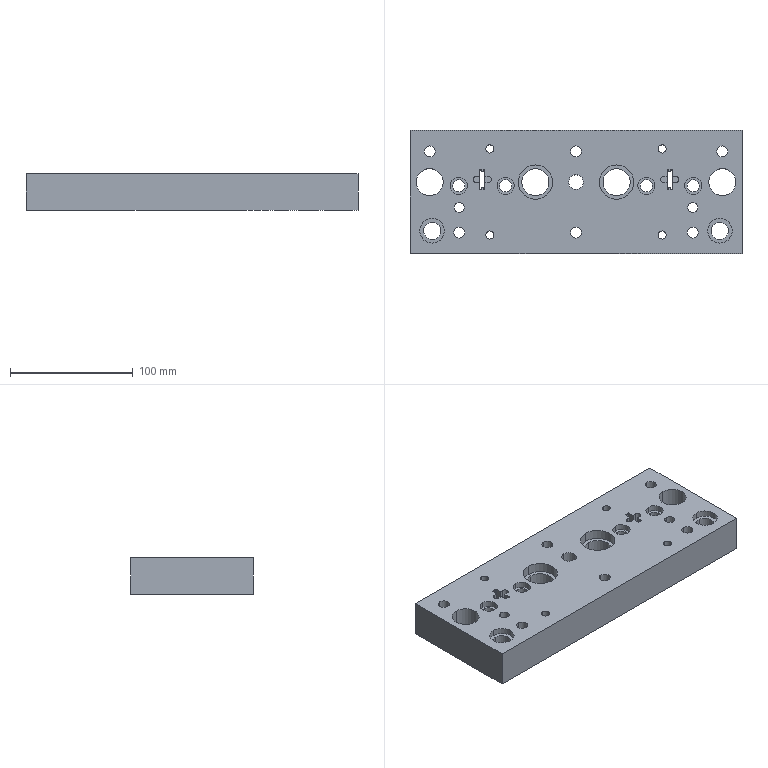Part | STEP file | TAM GA CHAY | 1 solid | 152 faces | box 270 x 100 x 30 mm | volume 706425 mm3 | cylinder 100 | plane 52 | commonest cylinder face diameters 0.4 x16 9 x12 14 x12 15 x12 6.647 x8 10 x8